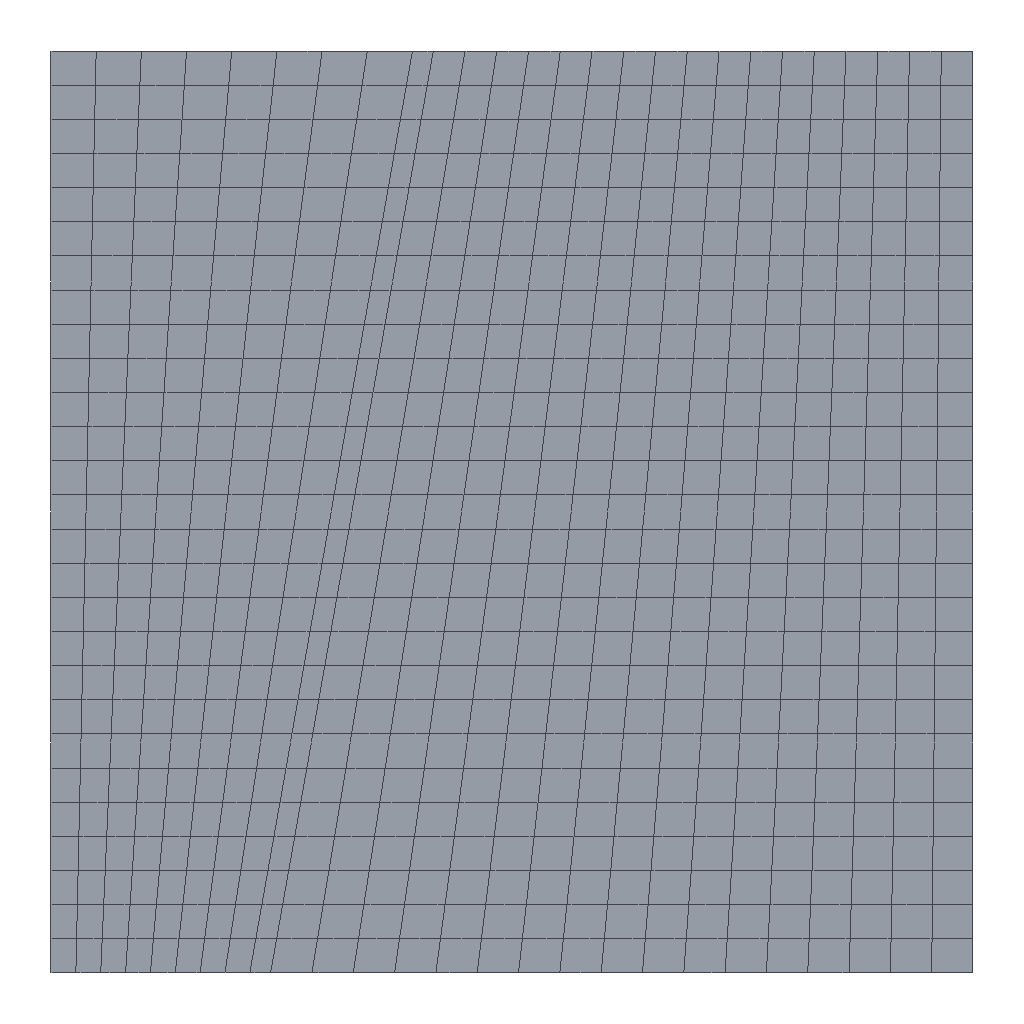Simulation study | abaqus
Set-up summary:
category,name,step,type,value,unit,region
solver,abaqus
solver,version,,,Abaqus/Standard 2020
units,not stated in the deck,,not stated
analysis,deck,,soils,soils
load_step,Step-1,Step-1,soils
load_step,requested,,,1
mesh,nodes,,,756
mesh,elements,,,702
element_type,CPE4P,,plane,702
load,load commands in deck,,count,3
bc,support commands in deck,,count,4
material,CHUSHUI,,in results
material,DUANCENG,,in results
material,SOIL,,in results
check,setup vs results,,match,"per instance, exact: element labels, types and connectivity; labels of the nodes the elements use; coordinates of those nodes at SINGLE_PRECISION in 1 of 1 instance(s)"
Abaqus input file, long lists of numbers shortened:
*Heading
** Job name: Job-1 Model name: Model-1
** Generated by: Abaqus/CAE 2020
*Preprint, echo=NO, model=NO, history=NO, contact=NO
**
** PARTS
**
*Part, name=Part-1
*Node
      1,   373.091,           0.
      2,   284.928,        -500.
** (754 more lines like these left out)
*Element, type=CPE4P
  1,   1,  17, 205,  76
  2,  17,  18, 206, 205
** (700 more lines like these left out)
*Nset, nset=Set-1
   9,  14, 176, 177
*Elset, elset=Set-1
 568, 569, 570, 590, 598, 606
*Nset, nset=Set-2
   1,   2,   3,   4,   5,   6,   7,   8,   9,  10,  11,  12,  13,  14,  15,  16
  17,  18,  19,  20,  21,  22,  23,  24,  25,  26,  27,  28,  29,  30,  31,  32
** (42 more lines like these left out)
*Elset, elset=Set-2
   1,   2,   3,   4,   5,   6,   7,   8,   9,  10,  11,  12,  13,  14,  15,  16
  17,  18,  19,  20,  21,  22,  23,  24,  25,  26,  27,  28,  29,  30,  31,  32
** (36 more lines like these left out)
*Nset, nset=Set-3
   2,   3,   5,   6,   9,  12,  14,  15,  31,  32,  33,  34,  35,  36,  37,  38
  39,  40,  41,  42,  43,  44,  45,  46,  77,  78,  79,  80,  81,  82,  83,  84
** (5 more lines like these left out)
*Elset, elset=Set-3
 256, 257, 258, 259, 260, 261, 262, 263, 264, 265, 266, 267, 268, 269, 270, 271
 272, 273, 274, 275, 276, 277, 278, 279, 280, 281, 282, 283, 284, 285, 286, 287
** (3 more lines like these left out)
*Nset, nset=Set-4
   1,   2,   5,   7,   9,  10,  13,  14,  17,  18,  19,  20,  21,  22,  23,  24
  25,  26,  27,  28,  29,  30,  95,  96,  97,  98,  99, 100, 101, 102, 103, 104
** (2 more lines like these left out)
*Elset, elset=Set-4, generate
 556,  582,    1
** Section: Section-soil
*Solid Section, elset=Set-2, material=soil
,
** Section: chushui
*Solid Section, elset=Set-3, material=chushui
,
** Section: duanceng
*Solid Section, elset=Set-4, material=duanceng
,
*End Part
**
**
** ASSEMBLY
**
*Assembly, name=Assembly
**
*Instance, name=Part-1-1, part=Part-1
*End Instance
**
*Nset, nset=Set-1, instance=Part-1-1
   1,   2,   3,   4,   5,   7,   8,   9,  10,  11,  31,  32,  33,  34,  35,  36
  37,  38,  39,  40,  41,  42,  43,  44,  45,  46,  61,  62,  63,  64,  65,  66
** (4 more lines like these left out)
*Elset, elset=Set-1, instance=Part-1-1
   1,  15,  16,  30,  31,  45,  46,  60,  61,  75,  76,  90,  91, 105, 106, 120
 121, 135, 136, 150, 151, 165, 166, 180, 181, 195, 196, 210, 211, 225, 226, 240
** (6 more lines like these left out)
*Nset, nset=Set-2, instance=Part-1-1
   1,   2,   3,   4,   5,   6,   7,  11,  12,  15,  16,  31,  32,  33,  34,  35
  36,  37,  38,  39,  40,  41,  42,  43,  44,  45,  46,  61,  62,  63,  64,  65
** (4 more lines like these left out)
*Elset, elset=Set-2, instance=Part-1-1
   1,  15,  16,  30,  31,  45,  46,  60,  61,  75,  76,  90,  91, 105, 106, 120
 121, 135, 136, 150, 151, 165, 166, 180, 181, 195, 196, 210, 211, 225, 226, 240
** (6 more lines like these left out)
*Nset, nset=Set-3, instance=Part-1-1
   1,   2,   5,  10,  11,  95,  96, 140, 141, 142, 143, 144, 145, 146
*Elset, elset=Set-3, instance=Part-1-1
 256, 273, 290, 471, 483, 495, 507, 519, 531, 543, 555, 565, 566, 567, 582
*Nset, nset=Set-4, instance=Part-1-1
   1,   2,   3,   4,   5,   6,   7,   8,   9,  10,  11,  31,  32,  33,  34,  35
  36,  37,  38,  39,  40,  41,  42,  43,  44,  45,  46,  61,  62,  63,  64,  65
** (3 more lines like these left out)
*Elset, elset=Set-4, instance=Part-1-1
   1,  15,  16,  30,  31,  45,  46,  60,  61,  75,  76,  90,  91, 105, 106, 120
 121, 135, 136, 150, 151, 165, 166, 180, 181, 195, 196, 210, 211, 225, 226, 240
** (5 more lines like these left out)
*Nset, nset=Set-5, instance=Part-1-1
   7,   9,  13,  14, 176, 177
*Elset, elset=Set-5, instance=Part-1-1
 556, 568, 569, 570, 590, 598, 606
*Nset, nset=Set-6, instance=Part-1-1
   3,   5,   6,  15,  16,  77,  78,  79,  80,  81,  82,  83,  84,  85,  86,  87
  88,  89,  90,  91,  92,  93,  94, 187, 188, 189, 190, 191, 192, 193, 194, 195
** (1 more lines like these left out)
*Elset, elset=Set-6, instance=Part-1-1
 256, 257, 258, 259, 260, 261, 262, 263, 264, 265, 266, 267, 268, 269, 270, 271
 272, 289, 306, 307, 316, 325, 334, 343, 352, 361, 370, 379, 388, 397, 406, 415
** (1 more lines like these left out)
*Nset, nset=Set-7, instance=Part-1-1, generate
   1,  756,    1
*Elset, elset=Set-7, instance=Part-1-1, generate
   1,  702,    1
*Nset, nset=Set-8, instance=Part-1-1
   3,   4,   6,   8,  11,  12,  15,  16,  47,  48,  49,  50,  51,  52,  53,  54
  55,  56,  57,  58,  59,  60,  93,  94, 121, 122, 123, 124, 125, 126, 127, 128
** (2 more lines like these left out)
*Elset, elset=Set-8, instance=Part-1-1
 241, 242, 243, 244, 245, 246, 247, 248, 249, 250, 251, 252, 253, 254, 255, 272
 289, 306, 451, 452, 453, 454, 455, 456, 457, 458, 459, 544, 545, 546, 547, 548
** (2 more lines like these left out)
*Nset, nset=Set-9, instance=Part-1-1
   7,   8,  13,  16, 105, 106, 107, 108, 109, 110, 111, 112, 113, 114, 115, 116
 117, 118, 119, 120, 198, 199, 200, 201, 202, 203, 204
*Elset, elset=Set-9, instance=Part-1-1
 315, 324, 333, 342, 351, 360, 369, 378, 387, 396, 405, 414, 423, 432, 441, 450
 459, 556, 695, 696, 697, 698, 699, 700, 701, 702
*Nset, nset=Set-10, instance=Part-1-1
   1,   4,  10,  11,  61,  62,  63,  64,  65,  66,  67,  68,  69,  70,  71,  72
  73,  74,  75,  76, 140, 141, 142, 143, 144, 145, 146
*Elset, elset=Set-10, instance=Part-1-1
   1,  16,  31,  46,  61,  76,  91, 106, 121, 136, 151, 166, 181, 196, 211, 226
 241, 471, 483, 495, 507, 519, 531, 543, 555, 582
*Nset, nset=Set-11, instance=Part-1-1
   9,  14, 176, 177
*Elset, elset=Set-11, instance=Part-1-1
 568, 569, 570, 590, 598, 606
*Nset, nset=Set-12, instance=Part-1-1, generate
   1,  756,    1
*Elset, elset=Set-12, instance=Part-1-1, generate
   1,  702,    1
*Nset, nset=Set-13, instance=Part-1-1
   9,  14, 176, 177
*Elset, elset=Set-13, instance=Part-1-1
 568, 569, 570, 590, 598, 606
*Nset, nset=Set-14, instance=Part-1-1
   1,   4,  10,  11,  61,  62,  63,  64,  65,  66,  67,  68,  69,  70,  71,  72
  73,  74,  75,  76, 140, 141, 142, 143, 144, 145, 146
*Elset, elset=Set-14, instance=Part-1-1
   1,  16,  31,  46,  61,  76,  91, 106, 121, 136, 151, 166, 181, 196, 211, 226
 241, 471, 483, 495, 507, 519, 531, 543, 555
*Nset, nset=Set-15, instance=Part-1-1
  1, 10
*Elset, elset=Set-15, instance=Part-1-1
 582,
*Nset, nset=Set-16, instance=Part-1-1
   1,   4,  10,  11,  61,  62,  63,  64,  65,  66,  67,  68,  69,  70,  71,  72
  73,  74,  75,  76, 140, 141, 142, 143, 144, 145, 146
*Elset, elset=Set-16, instance=Part-1-1
   1,  16,  31,  46,  61,  76,  91, 106, 121, 136, 151, 166, 181, 196, 211, 226
 241, 471, 483, 495, 507, 519, 531, 543, 555, 582
*Nset, nset=Set-17, instance=Part-1-1
  9, 14
*Nset, nset=Set-18, instance=Part-1-1
   1,   4,  10,  11,  61,  62,  63,  64,  65,  66,  67,  68,  69,  70,  71,  72
  73,  74,  75,  76, 140, 141, 142, 143, 144, 145, 146
*Elset, elset=Set-18, instance=Part-1-1
   1,  16,  31,  46,  61,  76,  91, 106, 121, 136, 151, 166, 181, 196, 211, 226
 241, 471, 483, 495, 507, 519, 531, 543, 555
*Nset, nset=Set-19, instance=Part-1-1
  1, 10
*Elset, elset=Set-19, instance=Part-1-1
 582,
*Nset, nset=Set-20, instance=Part-1-1
   4,  11,  61,  62,  63,  64,  65,  66,  67,  68,  69,  70,  71,  72,  73,  74
  75,  76, 140, 141, 142, 143, 144, 145, 146
*Elset, elset=Set-20, instance=Part-1-1
   1,  16,  31,  46,  61,  76,  91, 106, 121, 136, 151, 166, 181, 196, 211, 226
 241, 471, 483, 495, 507, 519, 531, 543, 555
*Nset, nset=Set-21, instance=Part-1-1
   2,   5,   9,  14,  95,  96, 176, 177
*Elset, elset=Set-21, instance=Part-1-1
 256, 273, 290, 565, 566, 567, 568, 569, 570, 590, 598, 606
*Nset, nset=Set-22, instance=Part-1-1
   4,  11,  61,  62,  63,  64,  65,  66,  67,  68,  69,  70,  71,  72,  73,  74
  75,  76, 140, 141, 142, 143, 144, 145, 146
*Elset, elset=Set-22, instance=Part-1-1
   1,  16,  31,  46,  61,  76,  91, 106, 121, 136, 151, 166, 181, 196, 211, 226
 241, 471, 483, 495, 507, 519, 531, 543, 555, 582
*Nset, nset=Set-23, instance=Part-1-1
   1,   4,  10,  11,  61,  62,  63,  64,  65,  66,  67,  68,  69,  70,  71,  72
  73,  74,  75,  76, 140, 141, 142, 143, 144, 145, 146
*Elset, elset=Set-23, instance=Part-1-1
   1,  16,  31,  46,  61,  76,  91, 106, 121, 136, 151, 166, 181, 196, 211, 226
 241, 471, 483, 495, 507, 519, 531, 543, 555, 582
*Nset, nset=Set-24, instance=Part-1-1
   1,   4,  10,  11,  61,  62,  63,  64,  65,  66,  67,  68,  69,  70,  71,  72
  73,  74,  75,  76, 140, 141, 142, 143, 144, 145, 146
*Elset, elset=Set-24, instance=Part-1-1
   1,  16,  31,  46,  61,  76,  91, 106, 121, 136, 151, 166, 181, 196, 211, 226
 241, 471, 483, 495, 507, 519, 531, 543, 555
*Nset, nset=Set-25, instance=Part-1-1
   4,  11,  61,  62,  63,  64,  65,  66,  67,  68,  69,  70,  71,  72,  73,  74
  75,  76, 140, 141, 142, 143, 144, 145, 146
*Elset, elset=Set-25, instance=Part-1-1
   1,  16,  31,  46,  61,  76,  91, 106, 121, 136, 151, 166, 181, 196, 211, 226
 241, 471, 483, 495, 507, 519, 531, 543, 555, 582
*Nset, nset=Set-26, instance=Part-1-1
   4,  11,  61,  62,  63,  64,  65,  66,  67,  68,  69,  70,  71,  72,  73,  74
  75,  76, 140, 141, 142, 143, 144, 145, 146
*Elset, elset=Set-26, instance=Part-1-1
   1,  16,  31,  46,  61,  76,  91, 106, 121, 136, 151, 166, 181, 196, 211, 226
 241, 471, 483, 495, 507, 519, 531, 543, 555
*Nset, nset=Set-27, instance=Part-1-1
   4,  11,  61,  62,  63,  64,  65,  66,  67,  68,  69,  70,  71,  72,  73,  74
  75,  76, 140, 141, 142, 143, 144, 145, 146
*Elset, elset=Set-27, instance=Part-1-1
   1,  16,  31,  46,  61,  76,  91, 106, 121, 136, 151, 166, 181, 196, 211, 226
 241, 471, 483, 495, 507, 519, 531, 543, 555, 582
*Elset, elset=_Surf-1_S2, internal, instance=Part-1-1
 272, 289, 306, 614, 622, 630, 638, 646, 654, 662, 670, 678, 686, 694, 702
*Elset, elset=_Surf-1_S1, internal, instance=Part-1-1, generate
 256,  272,    1
*Surface, type=ELEMENT, name=Surf-1
_Surf-1_S2, S2
_Surf-1_S1, S1
*Elset, elset=_Surf-2_S4, internal, instance=Part-1-1, generate
   1,  241,   15
*Elset, elset=_Surf-2_S2, internal, instance=Part-1-1, generate
 471,  555,   12
*Elset, elset=_Surf-2_S3, internal, instance=Part-1-1
 582,
*Surface, type=ELEMENT, name=Surf-2
_Surf-2_S4, S4
_Surf-2_S2, S2
_Surf-2_S3, S3
*Elset, elset=_Surf-3_S4, internal, instance=Part-1-1, generate
   1,  241,   15
*Elset, elset=_Surf-3_S2, internal, instance=Part-1-1, generate
 471,  555,   12
*Surface, type=ELEMENT, name=Surf-3
_Surf-3_S4, S4
_Surf-3_S2, S2
*Elset, elset=_Surf-4_S4, internal, instance=Part-1-1, generate
   1,  241,   15
*Elset, elset=_Surf-4_S2, internal, instance=Part-1-1, generate
 471,  555,   12
*Elset, elset=_Surf-4_S3, internal, instance=Part-1-1
 582,
*Surface, type=ELEMENT, name=Surf-4
_Surf-4_S4, S4
_Surf-4_S2, S2
_Surf-4_S3, S3
*Elset, elset=_Surf-5_S4, internal, instance=Part-1-1, generate
   1,  241,   15
*Elset, elset=_Surf-5_S2, internal, instance=Part-1-1, generate
 471,  555,   12
*Surface, type=ELEMENT, name=Surf-5
_Surf-5_S4, S4
_Surf-5_S2, S2
*Elset, elset=_Surf-6_S4, internal, instance=Part-1-1, generate
   1,  241,   15
*Elset, elset=_Surf-6_S2, internal, instance=Part-1-1, generate
 471,  555,   12
*Elset, elset=_Surf-6_S3, internal, instance=Part-1-1
 582,
*Surface, type=ELEMENT, name=Surf-6
_Surf-6_S4, S4
_Surf-6_S2, S2
_Surf-6_S3, S3
*Elset, elset=_Surf-7_S4, internal, instance=Part-1-1, generate
   1,  241,   15
*Elset, elset=_Surf-7_S2, internal, instance=Part-1-1, generate
 471,  555,   12
*Surface, type=ELEMENT, name=Surf-7
_Surf-7_S4, S4
_Surf-7_S2, S2
*Elset, elset=_Surf-8_S4, internal, instance=Part-1-1, generate
   1,  241,   15
*Elset, elset=_Surf-8_S2, internal, instance=Part-1-1, generate
 471,  555,   12
*Elset, elset=_Surf-8_S3, internal, instance=Part-1-1
 582,
*Surface, type=ELEMENT, name=Surf-8
_Surf-8_S4, S4
_Surf-8_S2, S2
_Surf-8_S3, S3
*Nset, nset=Set-21_PP_, internal, instance=Part-1-1
   2,   5,   9,  14,  95,  96, 176, 177
*Nset, nset=Set-27_PP_, internal, instance=Part-1-1
   4,  11,  61,  62,  63,  64,  65,  66,  67,  68,  69,  70,  71,  72,  73,  74
  75,  76, 140, 141, 142, 143, 144, 145, 146
*End Assembly
*Amplitude, name=Amp-1
             0.,              0.,              1.,              1.
**
** MATERIALS
**
*Material, name=chushui
*Density
2200.,
*Elastic
 1.44e+10, 0.2
*Gap Flow
 0.001,
*Permeability, specific=9980.
 1.5e-13, 0.19
*Material, name=duanceng
*Density
2200.,
*Elastic
 1.44e+10, 0.2
*Gap Flow
 0.001,
*Permeability, specific=9980.
 1.5e-09, 0.19
*Material, name=soil
*Density
2500.,
*Elastic
 2.964e+10, 0.12
*Gap Flow
 0.001,
*Permeability, specific=9980.
 2e-16, 0.04
**
** BOUNDARY CONDITIONS
**
** Name: BC-1 Type: 位移/转角
*Boundary
Set-8, 1, 1
** Name: BC-2 Type: 位移/转角
*Boundary
Set-9, 2, 2
**
** PREDEFINED FIELDS
**
** Name: Predefined Field-1   Type: Stress
*Initial Conditions, type=STRESS
Set-7, 0., 0., 0., 0.,
** Name: Predefined Field-2   Type: Void ratio
*Initial Conditions, TYPE=RATIO
Set-12, 1.
** ----------------------------------------------------------------
**
** STEP: Step-1
**
*Step, name=Step-1, nlgeom=YES, inc=1000
*Soils, utol=1.0, creep=none, stabilize=0.0002, allsdtol=0.05, continue=NO
0.01, 1., 1e-05, 1.,
**
** BOUNDARY CONDITIONS
**
** Name: BC-4 Type: 孔隙压力
*Boundary
Set-21_PP_, 8, 8, 1e+08
** Name: [REDACTED] : Pore pressure
*Boundary
Set-27_PP_, 8, 8, 3e+06
**
** LOADS
**
** Name: Load-pressure   Type: Pressure
*Dsload
Surf-8, P, 7.36e+06
**
** OUTPUT REQUESTS
**
*Restart, write, frequency=0
**
** FIELD OUTPUT: F-Output-1
**
*Output, field
*Node Output
CF, POR, RF, U, V
*Element Output, directions=YES
E, FLUVR, FLVEL, LE, MISES, MISESMAX, PE, S, SAT, VOIDR, PEEQ
*Contact Output
PFL, PFLA, PTL, PTLA
**
** HISTORY OUTPUT: H-Output-1
**
*Output, history, variable=PRESELECT
*End Step
Results summary:
result,step,,completed,increments=11 time=1.0/1.0
result,analysis,,,soils
result,last_loadstep,,,1
result,primary field,,,"U, POR"
result,reaction total,,FX,2000288.0,model units
result,reaction total,,FY,6624011427.0,model units
result,reaction total,,FZ,0.0,model units